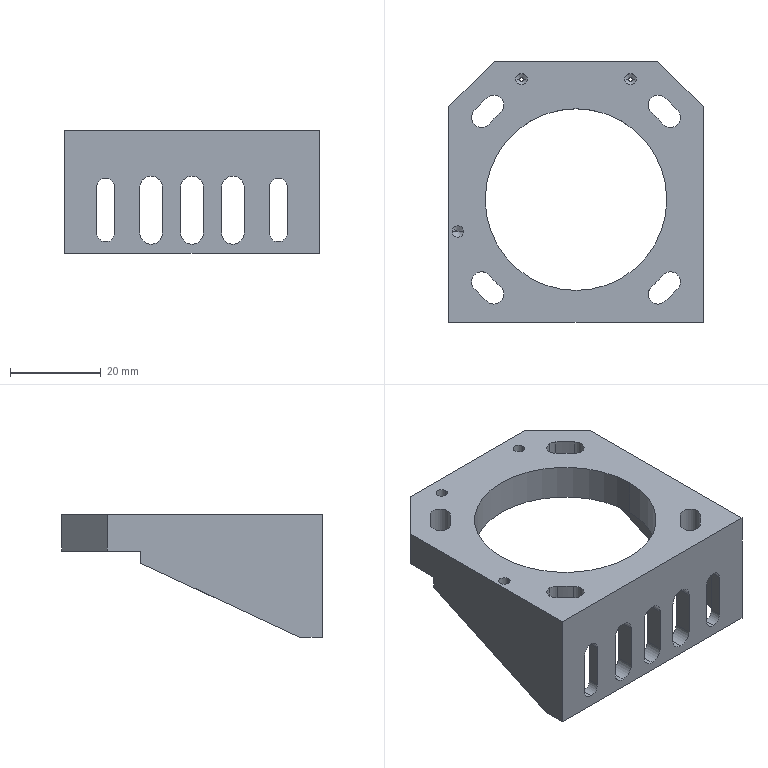NC program | NX | posted with a generic post | part box 56 x 57.4 x 27 mm
Lines 3844 to 3927 of 24340:
(ZLEVEL_PROFILE_COPY , TOOL : D10JING)
N7668 T11 M6
N7670 G54
N7672 G17 G0 G90 X-30.322 Y34.809 B0. C0. S5000 M3
N7674 G43 Z30. H11
N7676 Z-7.5
N7678 G94 G1 Z-9. F1000.
N7680 X-29.566 Y33.5
N7682 G3 X-28.7 Y33. R1.
N7684 G1 X18.7 F1200.
N7686 G2 X22.236 Y31.536 R5.
N7688 G1 X32.236 Y21.536
N7690 G2 X33.7 Y18. R5.
N7692 G1 Y-18.
N7694 G2 X32.236 Y-21.536 R5.
N7696 G1 X22.236 Y-31.536
N7698 G2 X18.7 Y-33. R5.
N7700 G1 X-28.7
N7702 G2 X-33.7 Y-28. R5.
N7704 G1 Y28.
N7706 G2 X-28.7 Y33. R5.
N7708 G3 X-27.834 Y33.5 R1.
N7710 G1 X-26.968 Y35.
N7712 Z-7.5
N7714 G0 Z3.
N7716 X-30.322 Y34.809
N7718 Z-16.5
N7720 G1 Z-18. F1000.
N7722 X-29.566 Y33.5
N7724 G3 X-28.7 Y33. R1.
N7726 G1 X18.7 F1200.
N7728 G2 X22.236 Y31.536 R5.
N7730 G1 X32.236 Y21.536
N7732 G2 X33.7 Y18. R5.
N7734 G1 Y-18.
N7736 G2 X32.236 Y-21.536 R5.
N7738 G1 X22.236 Y-31.536
N7740 G2 X18.7 Y-33. R5.
N7742 G1 X-28.7
N7744 G2 X-33.7 Y-28. R5.
N7746 G1 Y28.
N7748 G2 X-28.7 Y33. R5.
N7750 G3 X-27.834 Y33.5 R1.
N7752 G1 X-26.968 Y35.
N7754 Z-16.5
N7756 G0 Z-6.
N7758 X-30.322 Y34.809
N7760 Z-25.5
N7762 G1 Z-27. F1000.
N7764 X-29.566 Y33.5
N7766 G3 X-28.7 Y33. R1.
N7768 G1 X18.7 F1200.
N7770 G2 X22.236 Y31.536 R5.
N7772 G1 X32.236 Y21.536
N7774 G2 X33.7 Y18. R5.
N7776 G1 Y-18.
N7778 G2 X32.236 Y-21.536 R5.
N7780 G1 X22.236 Y-31.536
N7782 G2 X18.7 Y-33. R5.
N7784 G1 X-28.7
N7786 G2 X-33.7 Y-28. R5.
N7788 G1 Y28.
N7790 G2 X-28.7 Y33. R5.
N7792 G3 X-27.834 Y33.5 R1.
N7794 G1 X-26.968 Y35.
N7796 Z-25.5
N7798 G0 Z30.
(ZLEVEL_PROFILE_COPY_COPY , TOOL : D10JING)
N7800 X0.105 Y12.874
N7802 Z-6.5
N7804 G1 Z-8. F1000.
N7806 X-0.834 Y14.5
N7808 G3 X-1.7 Y15. R1.
N7810 X-16.7 Y0. R15. F1200.
N7812 X-1.7 Y15. R-15.
N7814 X-2.566 Y14.5 R1.
N7816 G1 X-3.505 Y12.874
N7818 Z-6.5
N7820 G0 Z30.
N7822 M5